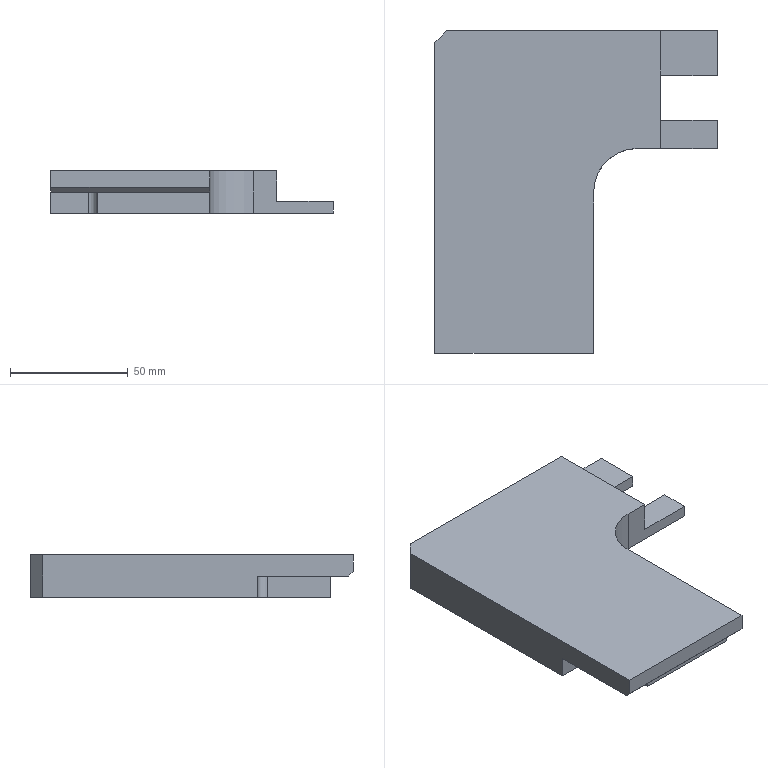Part | STEP file | PN_0038 | 1 solid | 28 faces | box 120 x 137 x 18 mm | volume 154666 mm3 | plane 23 | cylinder 5 | commonest cylinder face diameters 8 x1 19 x1 37 x1 61 x1 99 x1